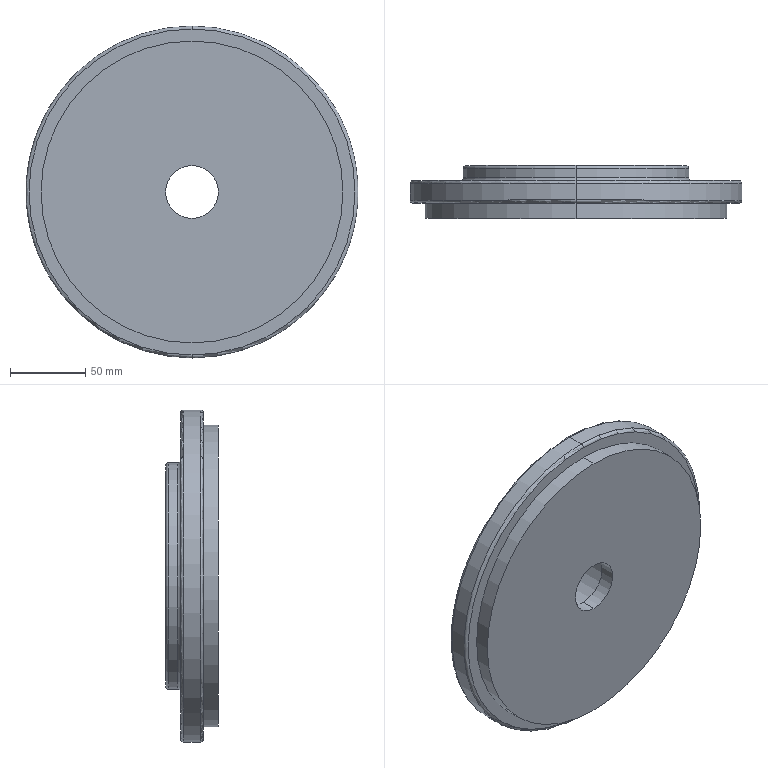Part | SolidWorks | features ICE 4, Fillet 2, CirPattern 1, Extrusion 1, HoleWzd 1 | 1 solid | 39 faces | box 220 x 35 x 220 mm | volume 996825 mm3 | cylinder 18 | torus 8 | cone 8 | plane 5 | commonest cylinder face diameters 3.3 x8 35 x2 52 x2 150 x2 200 x2 220 x2
STEP:
#1=CARTESIAN_POINT('',(0.,23.,-110.));
#2=VERTEX_POINT('',#1);
#3=CARTESIAN_POINT('',(0.,23.,110.));
#4=VERTEX_POINT('',#3);
#5=CARTESIAN_POINT('',(0.,23.,0.));
#6=DIRECTION('',(0.,-1.,0.));
#7=DIRECTION('',(0.,0.,1.));
#8=AXIS2_PLACEMENT_3D('',#5,#6,#7);
#9=CIRCLE('',#8,110.);
#10=EDGE_CURVE('',#2,#4,#9,.T.);
#11=ORIENTED_EDGE('',*,*,#10,.F.);
#12=CARTESIAN_POINT('',(0.,25.,-108.));
#13=VERTEX_POINT('',#12);
#14=CARTESIAN_POINT('',(0.,23.,-108.));
#15=DIRECTION('',(1.,0.,0.));
#16=DIRECTION('',(0.,0.,-1.));
#17=AXIS2_PLACEMENT_3D('',#14,#15,#16);
#18=CIRCLE('',#17,2.);
#19=EDGE_CURVE('',#2,#13,#18,.T.);
#20=ORIENTED_EDGE('',*,*,#19,.T.);
#21=CARTESIAN_POINT('',(0.,25.,108.));
#22=VERTEX_POINT('',#21);
#23=CARTESIAN_POINT('',(0.,25.,0.));
#24=DIRECTION('',(0.,1.,0.));
#25=DIRECTION('',(0.,0.,1.));
#26=AXIS2_PLACEMENT_3D('',#23,#24,#25);
#27=CIRCLE('',#26,108.);
#28=EDGE_CURVE('',#22,#13,#27,.T.);
#29=ORIENTED_EDGE('',*,*,#28,.F.);
#30=CARTESIAN_POINT('',(0.,23.,108.));
#31=DIRECTION('',(-1.,0.,0.));
#32=DIRECTION('',(0.,0.,1.));
#33=AXIS2_PLACEMENT_3D('',#30,#31,#32);
#34=CIRCLE('',#33,2.);
#35=EDGE_CURVE('',#4,#22,#34,.T.);
#36=ORIENTED_EDGE('',*,*,#35,.F.);
#37=EDGE_LOOP('',(#11,#20,#29,#36));
#38=FACE_OUTER_BOUND('',#37,.T.);
#39=CARTESIAN_POINT('',(0.,23.,0.));
#40=DIRECTION('',(0.,1.,0.));
#41=DIRECTION('',(0.,0.,1.));
#42=AXIS2_PLACEMENT_3D('',#39,#40,#41);
#43=TOROIDAL_SURFACE('',#42,108.,2.);
#44=ADVANCED_FACE('',(#38),#43,.T.);
#45=CARTESIAN_POINT('',(0.,10.,-108.));
#46=VERTEX_POINT('',#45);
#47=CARTESIAN_POINT('',(0.,10.,108.));
#48=VERTEX_POINT('',#47);
#49=CARTESIAN_POINT('',(0.,10.,0.));
#50=DIRECTION('',(0.,-1.,0.));
#51=DIRECTION('',(0.,0.,1.));
#52=AXIS2_PLACEMENT_3D('',#49,#50,#51);
#53=CIRCLE('',#52,108.);
#54=EDGE_CURVE('',#46,#48,#53,.T.);
#55=ORIENTED_EDGE('',*,*,#54,.F.);
#56=CARTESIAN_POINT('',(0.,12.,-110.));
#57=VERTEX_POINT('',#56);
#58=CARTESIAN_POINT('',(0.,12.,-108.));
#59=DIRECTION('',(1.,0.,0.));
#60=DIRECTION('',(0.,0.,-1.));
#61=AXIS2_PLACEMENT_3D('',#58,#59,#60);
#62=CIRCLE('',#61,2.);
#63=EDGE_CURVE('',#46,#57,#62,.T.);
#64=ORIENTED_EDGE('',*,*,#63,.T.);
#65=CARTESIAN_POINT('',(0.,12.,110.));
#66=VERTEX_POINT('',#65);
#67=CARTESIAN_POINT('',(0.,12.,0.));
#68=DIRECTION('',(0.,1.,0.));
#69=DIRECTION('',(0.,0.,1.));
#70=AXIS2_PLACEMENT_3D('',#67,#68,#69);
#71=CIRCLE('',#70,110.);
#72=EDGE_CURVE('',#66,#57,#71,.T.);
#73=ORIENTED_EDGE('',*,*,#72,.F.);
#74=CARTESIAN_POINT('',(0.,12.,108.));
#75=DIRECTION('',(-1.,0.,0.));
#76=DIRECTION('',(0.,0.,1.));
#77=AXIS2_PLACEMENT_3D('',#74,#75,#76);
#78=CIRCLE('',#77,2.);
#79=EDGE_CURVE('',#48,#66,#78,.T.);
#80=ORIENTED_EDGE('',*,*,#79,.F.);
#81=EDGE_LOOP('',(#55,#64,#73,#80));
#82=FACE_OUTER_BOUND('',#81,.T.);
#83=CARTESIAN_POINT('',(0.,12.,0.));
#84=DIRECTION('',(0.,1.,0.));
#85=DIRECTION('',(0.,0.,1.));
#86=AXIS2_PLACEMENT_3D('',#83,#84,#85);
#87=TOROIDAL_SURFACE('',#86,108.,2.);
#88=ADVANCED_FACE('',(#82),#87,.T.);
#89=CARTESIAN_POINT('',(30.,24.9,-1.65));
#90=VERTEX_POINT('',#89);
#91=CARTESIAN_POINT('',(30.,24.9,1.65));
#92=VERTEX_POINT('',#91);
#93=CARTESIAN_POINT('',(30.,24.9,0.));
#94=DIRECTION('',(0.,1.,0.));
#95=DIRECTION('',(0.,0.,1.));
#96=AXIS2_PLACEMENT_3D('',#93,#94,#95);
#97=CIRCLE('',#96,1.65);
#98=EDGE_CURVE('',#90,#92,#97,.T.);
#99=ORIENTED_EDGE('',*,*,#98,.F.);
#100=CARTESIAN_POINT('',(30.,35.,-1.65));
#101=VERTEX_POINT('',#100);
#102=CARTESIAN_POINT('',(30.,35.,-1.65));
#103=DIRECTION('',(0.,1.,0.));
#104=VECTOR('',#103,1000.);
#105=LINE('',#102,#104);
#106=EDGE_CURVE('',#90,#101,#105,.T.);
#107=ORIENTED_EDGE('',*,*,#106,.T.);
#108=CARTESIAN_POINT('',(30.,35.,1.65));
#109=VERTEX_POINT('',#108);
#110=CARTESIAN_POINT('',(30.,35.,0.));
#111=DIRECTION('',(0.,1.,0.));
#112=DIRECTION('',(0.,0.,1.));
#113=AXIS2_PLACEMENT_3D('',#110,#111,#112);
#114=CIRCLE('',#113,1.65);
#115=EDGE_CURVE('',#101,#109,#114,.T.);
#116=ORIENTED_EDGE('',*,*,#115,.T.);
#117=CARTESIAN_POINT('',(30.,35.,1.65));
#118=DIRECTION('',(0.,1.,0.));
#119=VECTOR('',#118,1000.);
#120=LINE('',#117,#119);
#121=EDGE_CURVE('',#92,#109,#120,.T.);
#122=ORIENTED_EDGE('',*,*,#121,.F.);
#123=EDGE_LOOP('',(#99,#107,#116,#122));
#124=FACE_OUTER_BOUND('',#123,.T.);
#125=CARTESIAN_POINT('',(30.,35.,0.));
#126=DIRECTION('',(0.,1.,0.));
#127=DIRECTION('',(0.,0.,1.));
#128=AXIS2_PLACEMENT_3D('',#125,#126,#127);
#129=CYLINDRICAL_SURFACE('',#128,1.65);
#130=ADVANCED_FACE('',(#124),#129,.F.);
#131=CARTESIAN_POINT('',(30.,23.909,0.));
#132=VERTEX_POINT('',#131);
#133=CARTESIAN_POINT('',(30.,24.9,1.65));
#134=DIRECTION('',(0.,0.515,0.8572));
#135=VECTOR('',#134,1000.);
#136=LINE('',#133,#135);
#137=EDGE_CURVE('',#132,#92,#136,.T.);
#138=ORIENTED_EDGE('',*,*,#137,.F.);
#139=CARTESIAN_POINT('',(30.,24.9,-1.65));
#140=DIRECTION('',(0.,0.515,-0.8572));
#141=VECTOR('',#140,1000.);
#142=LINE('',#139,#141);
#143=EDGE_CURVE('',#132,#90,#142,.T.);
#144=ORIENTED_EDGE('',*,*,#143,.T.);
#145=ORIENTED_EDGE('',*,*,#98,.T.);
#146=EDGE_LOOP('',(#138,#144,#145));
#147=FACE_OUTER_BOUND('',#146,.T.);
#148=CARTESIAN_POINT('',(30.,24.9,0.));
#149=DIRECTION('',(0.,1.,0.));
#150=DIRECTION('',(0.,0.,1.));
#151=AXIS2_PLACEMENT_3D('',#148,#149,#150);
#152=CONICAL_SURFACE('',#151,1.65,1.03);
#153=ADVANCED_FACE('',(#147),#152,.F.);
#154=CARTESIAN_POINT('',(0.,24.9,28.35));
#155=VERTEX_POINT('',#154);
#156=CARTESIAN_POINT('',(0.,24.9,31.65));
#157=VERTEX_POINT('',#156);
#158=CARTESIAN_POINT('',(0.,24.9,30.));
#159=DIRECTION('',(0.,1.,0.));
#160=DIRECTION('',(0.,0.,1.));
#161=AXIS2_PLACEMENT_3D('',#158,#159,#160);
#162=CIRCLE('',#161,1.65);
#163=EDGE_CURVE('',#155,#157,#162,.T.);
#164=ORIENTED_EDGE('',*,*,#163,.F.);
#165=CARTESIAN_POINT('',(0.,35.,28.35));
#166=VERTEX_POINT('',#165);
#167=CARTESIAN_POINT('',(0.,35.,28.35));
#168=DIRECTION('',(0.,1.,0.));
#169=VECTOR('',#168,1000.);
#170=LINE('',#167,#169);
#171=EDGE_CURVE('',#155,#166,#170,.T.);
#172=ORIENTED_EDGE('',*,*,#171,.T.);
#173=CARTESIAN_POINT('',(0.,35.,31.65));
#174=VERTEX_POINT('',#173);
#175=CARTESIAN_POINT('',(0.,35.,30.));
#176=DIRECTION('',(0.,1.,0.));
#177=DIRECTION('',(0.,0.,1.));
#178=AXIS2_PLACEMENT_3D('',#175,#176,#177);
#179=CIRCLE('',#178,1.65);
#180=EDGE_CURVE('',#166,#174,#179,.T.);
#181=ORIENTED_EDGE('',*,*,#180,.T.);
#182=CARTESIAN_POINT('',(0.,35.,31.65));
#183=DIRECTION('',(0.,1.,0.));
#184=VECTOR('',#183,1000.);
#185=LINE('',#182,#184);
#186=EDGE_CURVE('',#157,#174,#185,.T.);
#187=ORIENTED_EDGE('',*,*,#186,.F.);
#188=EDGE_LOOP('',(#164,#172,#181,#187));
#189=FACE_OUTER_BOUND('',#188,.T.);
#190=CARTESIAN_POINT('',(0.,35.,30.));
#191=DIRECTION('',(0.,1.,0.));
#192=DIRECTION('',(0.,0.,1.));
#193=AXIS2_PLACEMENT_3D('',#190,#191,#192);
#194=CYLINDRICAL_SURFACE('',#193,1.65);
#195=ADVANCED_FACE('',(#189),#194,.F.);
#196=CARTESIAN_POINT('',(0.,23.909,30.));
#197=VERTEX_POINT('',#196);
#198=CARTESIAN_POINT('',(0.,24.9,31.65));
#199=DIRECTION('',(0.,0.515,0.8572));
#200=VECTOR('',#199,1000.);
#201=LINE('',#198,#200);
#202=EDGE_CURVE('',#197,#157,#201,.T.);
#203=ORIENTED_EDGE('',*,*,#202,.F.);
#204=CARTESIAN_POINT('',(0.,24.9,28.35));
#205=DIRECTION('',(0.,0.515,-0.8572));
#206=VECTOR('',#205,1000.);
#207=LINE('',#204,#206);
#208=EDGE_CURVE('',#197,#155,#207,.T.);
#209=ORIENTED_EDGE('',*,*,#208,.T.);
#210=ORIENTED_EDGE('',*,*,#163,.T.);
#211=EDGE_LOOP('',(#203,#209,#210));
#212=FACE_OUTER_BOUND('',#211,.T.);
#213=CARTESIAN_POINT('',(0.,24.9,30.));
#214=DIRECTION('',(0.,1.,0.));
#215=DIRECTION('',(0.,0.,1.));
#216=AXIS2_PLACEMENT_3D('',#213,#214,#215);
#217=CONICAL_SURFACE('',#216,1.65,1.03);
#218=ADVANCED_FACE('',(#212),#217,.F.);
#219=CARTESIAN_POINT('',(-30.,24.9,-1.65));
#220=VERTEX_POINT('',#219);
#221=CARTESIAN_POINT('',(-30.,24.9,1.65));
#222=VERTEX_POINT('',#221);
#223=CARTESIAN_POINT('',(-30.,24.9,0.));
#224=DIRECTION('',(0.,1.,0.));
#225=DIRECTION('',(0.,0.,1.));
#226=AXIS2_PLACEMENT_3D('',#223,#224,#225);
#227=CIRCLE('',#226,1.65);
#228=EDGE_CURVE('',#220,#222,#227,.T.);
#229=ORIENTED_EDGE('',*,*,#228,.F.);
#230=CARTESIAN_POINT('',(-30.,35.,-1.65));
#231=VERTEX_POINT('',#230);
#232=CARTESIAN_POINT('',(-30.,35.,-1.65));
#233=DIRECTION('',(0.,1.,0.));
#234=VECTOR('',#233,1000.);
#235=LINE('',#232,#234);
#236=EDGE_CURVE('',#220,#231,#235,.T.);
#237=ORIENTED_EDGE('',*,*,#236,.T.);
#238=CARTESIAN_POINT('',(-30.,35.,1.65));
#239=VERTEX_POINT('',#238);
#240=CARTESIAN_POINT('',(-30.,35.,0.));
#241=DIRECTION('',(0.,1.,0.));
#242=DIRECTION('',(0.,0.,1.));
#243=AXIS2_PLACEMENT_3D('',#240,#241,#242);
#244=CIRCLE('',#243,1.65);
#245=EDGE_CURVE('',#231,#239,#244,.T.);
#246=ORIENTED_EDGE('',*,*,#245,.T.);
#247=CARTESIAN_POINT('',(-30.,35.,1.65));
#248=DIRECTION('',(0.,1.,0.));
#249=VECTOR('',#248,1000.);
#250=LINE('',#247,#249);
#251=EDGE_CURVE('',#222,#239,#250,.T.);
#252=ORIENTED_EDGE('',*,*,#251,.F.);
#253=EDGE_LOOP('',(#229,#237,#246,#252));
#254=FACE_OUTER_BOUND('',#253,.T.);
#255=CARTESIAN_POINT('',(-30.,35.,0.));
#256=DIRECTION('',(0.,1.,0.));
#257=DIRECTION('',(0.,0.,1.));
#258=AXIS2_PLACEMENT_3D('',#255,#256,#257);
#259=CYLINDRICAL_SURFACE('',#258,1.65);
#260=ADVANCED_FACE('',(#254),#259,.F.);
#261=CARTESIAN_POINT('',(-30.,23.909,0.));
#262=VERTEX_POINT('',#261);
#263=CARTESIAN_POINT('',(-30.,24.9,1.65));
#264=DIRECTION('',(0.,0.515,0.8572));
#265=VECTOR('',#264,1000.);
#266=LINE('',#263,#265);
#267=EDGE_CURVE('',#262,#222,#266,.T.);
#268=ORIENTED_EDGE('',*,*,#267,.F.);
#269=CARTESIAN_POINT('',(-30.,24.9,-1.65));
#270=DIRECTION('',(0.,0.515,-0.8572));
#271=VECTOR('',#270,1000.);
#272=LINE('',#269,#271);
#273=EDGE_CURVE('',#262,#220,#272,.T.);
#274=ORIENTED_EDGE('',*,*,#273,.T.);
#275=ORIENTED_EDGE('',*,*,#228,.T.);
#276=EDGE_LOOP('',(#268,#274,#275));
#277=FACE_OUTER_BOUND('',#276,.T.);
#278=CARTESIAN_POINT('',(-30.,24.9,0.));
#279=DIRECTION('',(0.,1.,0.));
#280=DIRECTION('',(0.,0.,1.));
#281=AXIS2_PLACEMENT_3D('',#278,#279,#280);
#282=CONICAL_SURFACE('',#281,1.65,1.03);
#283=ADVANCED_FACE('',(#277),#282,.F.);
#284=CARTESIAN_POINT('',(0.,24.9,-31.65));
#285=VERTEX_POINT('',#284);
#286=CARTESIAN_POINT('',(0.,24.9,-28.35));
#287=VERTEX_POINT('',#286);
#288=CARTESIAN_POINT('',(0.,24.9,-30.));
#289=DIRECTION('',(0.,1.,0.));
#290=DIRECTION('',(0.,0.,1.));
#291=AXIS2_PLACEMENT_3D('',#288,#289,#290);
#292=CIRCLE('',#291,1.65);
#293=EDGE_CURVE('',#285,#287,#292,.T.);
#294=ORIENTED_EDGE('',*,*,#293,.F.);
#295=CARTESIAN_POINT('',(0.,35.,-31.65));
#296=VERTEX_POINT('',#295);
#297=CARTESIAN_POINT('',(0.,35.,-31.65));
#298=DIRECTION('',(0.,1.,0.));
#299=VECTOR('',#298,1000.);
#300=LINE('',#297,#299);
#301=EDGE_CURVE('',#285,#296,#300,.T.);
#302=ORIENTED_EDGE('',*,*,#301,.T.);
#303=CARTESIAN_POINT('',(0.,35.,-28.35));
#304=VERTEX_POINT('',#303);
#305=CARTESIAN_POINT('',(0.,35.,-30.));
#306=DIRECTION('',(0.,1.,0.));
#307=DIRECTION('',(0.,0.,1.));
#308=AXIS2_PLACEMENT_3D('',#305,#306,#307);
#309=CIRCLE('',#308,1.65);
#310=EDGE_CURVE('',#296,#304,#309,.T.);
#311=ORIENTED_EDGE('',*,*,#310,.T.);
#312=CARTESIAN_POINT('',(0.,35.,-28.35));
#313=DIRECTION('',(0.,1.,0.));
#314=VECTOR('',#313,1000.);
#315=LINE('',#312,#314);
#316=EDGE_CURVE('',#287,#304,#315,.T.);
#317=ORIENTED_EDGE('',*,*,#316,.F.);
#318=EDGE_LOOP('',(#294,#302,#311,#317));
#319=FACE_OUTER_BOUND('',#318,.T.);
#320=CARTESIAN_POINT('',(0.,35.,-30.));
#321=DIRECTION('',(0.,1.,0.));
#322=DIRECTION('',(0.,0.,1.));
#323=AXIS2_PLACEMENT_3D('',#320,#321,#322);
#324=CYLINDRICAL_SURFACE('',#323,1.65);
#325=ADVANCED_FACE('',(#319),#324,.F.);
#326=CARTESIAN_POINT('',(0.,23.909,-30.));
#327=VERTEX_POINT('',#326);
#328=CARTESIAN_POINT('',(0.,24.9,-28.35));
#329=DIRECTION('',(0.,0.515,0.8572));
#330=VECTOR('',#329,1000.);
#331=LINE('',#328,#330);
#332=EDGE_CURVE('',#327,#287,#331,.T.);
#333=ORIENTED_EDGE('',*,*,#332,.F.);
#334=CARTESIAN_POINT('',(0.,24.9,-31.65));
#335=DIRECTION('',(0.,0.515,-0.8572));
#336=VECTOR('',#335,1000.);
#337=LINE('',#334,#336);
#338=EDGE_CURVE('',#327,#285,#337,.T.);
#339=ORIENTED_EDGE('',*,*,#338,.T.);
#340=ORIENTED_EDGE('',*,*,#293,.T.);
#341=EDGE_LOOP('',(#333,#339,#340));
#342=FACE_OUTER_BOUND('',#341,.T.);
#343=CARTESIAN_POINT('',(0.,24.9,-30.));
#344=DIRECTION('',(0.,1.,0.));
#345=DIRECTION('',(0.,0.,1.));
#346=AXIS2_PLACEMENT_3D('',#343,#344,#345);
#347=CONICAL_SURFACE('',#346,1.65,1.03);
#348=ADVANCED_FACE('',(#342),#347,.F.);
#349=CARTESIAN_POINT('',(0.,0.,-17.5));
#350=VERTEX_POINT('',#349);
#351=CARTESIAN_POINT('',(0.,0.,17.5));
#352=VERTEX_POINT('',#351);
#353=CARTESIAN_POINT('',(0.,0.,0.));
#354=DIRECTION('',(0.,1.,0.));
#355=DIRECTION('',(0.,0.,1.));
#356=AXIS2_PLACEMENT_3D('',#353,#354,#355);
#357=CIRCLE('',#356,17.5);
#358=EDGE_CURVE('',#350,#352,#357,.T.);
#359=ORIENTED_EDGE('',*,*,#358,.F.);
#360=CARTESIAN_POINT('',(0.,10.,-17.5));
#361=VERTEX_POINT('',#360);
#362=CARTESIAN_POINT('',(0.,0.,-17.5));
#363=DIRECTION('',(0.,1.,0.));
#364=VECTOR('',#363,1000.);
#365=LINE('',#362,#364);
#366=EDGE_CURVE('',#350,#361,#365,.T.);
#367=ORIENTED_EDGE('',*,*,#366,.T.);
#368=CARTESIAN_POINT('',(0.,10.,17.5));
#369=VERTEX_POINT('',#368);
#370=CARTESIAN_POINT('',(0.,10.,0.));
#371=DIRECTION('',(0.,1.,0.));
#372=DIRECTION('',(0.,0.,1.));
#373=AXIS2_PLACEMENT_3D('',#370,#371,#372);
#374=CIRCLE('',#373,17.5);
#375=EDGE_CURVE('',#361,#369,#374,.T.);
#376=ORIENTED_EDGE('',*,*,#375,.T.);
#377=CARTESIAN_POINT('',(0.,0.,17.5));
#378=DIRECTION('',(0.,1.,0.));
#379=VECTOR('',#378,1000.);
#380=LINE('',#377,#379);
#381=EDGE_CURVE('',#352,#369,#380,.T.);
#382=ORIENTED_EDGE('',*,*,#381,.F.);
#383=EDGE_LOOP('',(#359,#367,#376,#382));
#384=FACE_OUTER_BOUND('',#383,.T.);
#385=CARTESIAN_POINT('',(0.,0.,0.));
#386=DIRECTION('',(0.,1.,0.));
#387=DIRECTION('',(0.,0.,1.));
#388=AXIS2_PLACEMENT_3D('',#385,#386,#387);
#389=CYLINDRICAL_SURFACE('',#388,17.5);
#390=ADVANCED_FACE('',(#384),#389,.F.);
#391=CARTESIAN_POINT('',(0.,10.,-26.));
#392=VERTEX_POINT('',#391);
#393=CARTESIAN_POINT('',(0.,10.,26.));
#394=VERTEX_POINT('',#393);
#395=CARTESIAN_POINT('',(0.,10.,0.));
#396=DIRECTION('',(0.,1.,0.));
#397=DIRECTION('',(0.,0.,1.));
#398=AXIS2_PLACEMENT_3D('',#395,#396,#397);
#399=CIRCLE('',#398,26.);
#400=EDGE_CURVE('',#392,#394,#399,.T.);
#401=ORIENTED_EDGE('',*,*,#400,.F.);
#402=CARTESIAN_POINT('',(0.,35.,-26.));
#403=VERTEX_POINT('',#402);
#404=CARTESIAN_POINT('',(0.,10.,-26.));
#405=DIRECTION('',(0.,1.,0.));
#406=VECTOR('',#405,1000.);
#407=LINE('',#404,#406);
#408=EDGE_CURVE('',#392,#403,#407,.T.);
#409=ORIENTED_EDGE('',*,*,#408,.T.);
#410=CARTESIAN_POINT('',(0.,35.,26.));
#411=VERTEX_POINT('',#410);
#412=CARTESIAN_POINT('',(0.,35.,0.));
#413=DIRECTION('',(0.,1.,0.));
#414=DIRECTION('',(0.,0.,1.));
#415=AXIS2_PLACEMENT_3D('',#412,#413,#414);
#416=CIRCLE('',#415,26.);
#417=EDGE_CURVE('',#403,#411,#416,.T.);
#418=ORIENTED_EDGE('',*,*,#417,.T.);
#419=CARTESIAN_POINT('',(0.,10.,26.));
#420=DIRECTION('',(0.,1.,0.));
#421=VECTOR('',#420,1000.);
#422=LINE('',#419,#421);
#423=EDGE_CURVE('',#394,#411,#422,.T.);
#424=ORIENTED_EDGE('',*,*,#423,.F.);
#425=EDGE_LOOP('',(#401,#409,#418,#424));
#426=FACE_OUTER_BOUND('',#425,.T.);
#427=CARTESIAN_POINT('',(0.,10.,0.));
#428=DIRECTION('',(0.,1.,0.));
#429=DIRECTION('',(0.,0.,1.));
#430=AXIS2_PLACEMENT_3D('',#427,#428,#429);
#431=CYLINDRICAL_SURFACE('',#430,26.);
#432=ADVANCED_FACE('',(#426),#431,.F.);
#433=CARTESIAN_POINT('',(0.,27.,-75.));
#434=VERTEX_POINT('',#433);
#435=CARTESIAN_POINT('',(0.,27.,75.));
#436=VERTEX_POINT('',#435);
#437=CARTESIAN_POINT('',(0.,27.,0.));
#438=DIRECTION('',(0.,1.,0.));
#439=DIRECTION('',(0.,0.,1.));
#440=AXIS2_PLACEMENT_3D('',#437,#438,#439);
#441=CIRCLE('',#440,75.);
#442=EDGE_CURVE('',#434,#436,#441,.T.);
#443=ORIENTED_EDGE('',*,*,#442,.F.);
#444=CARTESIAN_POINT('',(0.,25.,-77.));
#445=VERTEX_POINT('',#444);
#446=CARTESIAN_POINT('',(0.,27.,-77.));
#447=DIRECTION('',(1.,0.,0.));
#448=DIRECTION('',(0.,0.,-1.));
#449=AXIS2_PLACEMENT_3D('',#446,#447,#448);
#450=CIRCLE('',#449,2.);
#451=EDGE_CURVE('',#434,#445,#450,.T.);
#452=ORIENTED_EDGE('',*,*,#451,.T.);
#453=CARTESIAN_POINT('',(0.,25.,77.));
#454=VERTEX_POINT('',#453);
#455=CARTESIAN_POINT('',(0.,25.,0.));
#456=DIRECTION('',(0.,-1.,0.));
#457=DIRECTION('',(0.,0.,1.));
#458=AXIS2_PLACEMENT_3D('',#455,#456,#457);
#459=CIRCLE('',#458,77.);
#460=EDGE_CURVE('',#454,#445,#459,.T.);
#461=ORIENTED_EDGE('',*,*,#460,.F.);
#462=CARTESIAN_POINT('',(0.,27.,77.));
#463=DIRECTION('',(-1.,0.,0.));
#464=DIRECTION('',(0.,0.,1.));
#465=AXIS2_PLACEMENT_3D('',#462,#463,#464);
#466=CIRCLE('',#465,2.);
#467=EDGE_CURVE('',#436,#454,#466,.T.);
#468=ORIENTED_EDGE('',*,*,#467,.F.);
#469=EDGE_LOOP('',(#443,#452,#461,#468));
#470=FACE_OUTER_BOUND('',#469,.T.);
#471=CARTESIAN_POINT('',(0.,27.,0.));
#472=DIRECTION('',(0.,1.,0.));
#473=DIRECTION('',(0.,0.,1.));
#474=AXIS2_PLACEMENT_3D('',#471,#472,#473);
#475=TOROIDAL_SURFACE('',#474,77.,2.);
#476=ADVANCED_FACE('',(#470),#475,.F.);
#477=CARTESIAN_POINT('',(0.,33.,-75.));
#478=VERTEX_POINT('',#477);
#479=CARTESIAN_POINT('',(0.,33.,75.));
#480=VERTEX_POINT('',#479);
#481=CARTESIAN_POINT('',(0.,33.,0.));
#482=DIRECTION('',(0.,-1.,0.));
#483=DIRECTION('',(0.,0.,1.));
#484=AXIS2_PLACEMENT_3D('',#481,#482,#483);
#485=CIRCLE('',#484,75.);
#486=EDGE_CURVE('',#478,#480,#485,.T.);
#487=ORIENTED_EDGE('',*,*,#486,.F.);
#488=CARTESIAN_POINT('',(0.,35.,-73.));
#489=VERTEX_POINT('',#488);
#490=CARTESIAN_POINT('',(0.,33.,-73.));
#491=DIRECTION('',(1.,0.,0.));
#492=DIRECTION('',(0.,0.,-1.));
#493=AXIS2_PLACEMENT_3D('',#490,#491,#492);
#494=CIRCLE('',#493,2.);
#495=EDGE_CURVE('',#478,#489,#494,.T.);
#496=ORIENTED_EDGE('',*,*,#495,.T.);
#497=CARTESIAN_POINT('',(0.,35.,73.));
#498=VERTEX_POINT('',#497);
#499=CARTESIAN_POINT('',(0.,35.,0.));
#500=DIRECTION('',(0.,1.,0.));
#501=DIRECTION('',(0.,0.,1.));
#502=AXIS2_PLACEMENT_3D('',#499,#500,#501);
#503=CIRCLE('',#502,73.);
#504=EDGE_CURVE('',#498,#489,#503,.T.);
#505=ORIENTED_EDGE('',*,*,#504,.F.);
#506=CARTESIAN_POINT('',(0.,33.,73.));
#507=DIRECTION('',(-1.,0.,0.));
#508=DIRECTION('',(0.,0.,1.));
#509=AXIS2_PLACEMENT_3D('',#506,#507,#508);
#510=CIRCLE('',#509,2.);
#511=EDGE_CURVE('',#480,#498,#510,.T.);
#512=ORIENTED_EDGE('',*,*,#511,.F.);
#513=EDGE_LOOP('',(#487,#496,#505,#512));
#514=FACE_OUTER_BOUND('',#513,.T.);
#515=CARTESIAN_POINT('',(0.,33.,0.));
#516=DIRECTION('',(0.,1.,0.));
#517=DIRECTION('',(0.,0.,1.));
#518=AXIS2_PLACEMENT_3D('',#515,#516,#517);
#519=TOROIDAL_SURFACE('',#518,73.,2.);
#520=ADVANCED_FACE('',(#514),#519,.T.);
#521=ORIENTED_EDGE('',*,*,#486,.T.);
#522=CARTESIAN_POINT('',(0.,35.,75.));
#523=DIRECTION('',(0.,-1.,0.));
#524=VECTOR('',#523,1000.);
#525=LINE('',#522,#524);
#526=EDGE_CURVE('',#480,#436,#525,.T.);
#527=ORIENTED_EDGE('',*,*,#526,.T.);
#528=CARTESIAN_POINT('',(0.,27.,0.));
#529=DIRECTION('',(0.,1.,0.));
#530=DIRECTION('',(0.,0.,1.));
#531=AXIS2_PLACEMENT_3D('',#528,#529,#530);
#532=CIRCLE('',#531,75.);
#533=EDGE_CURVE('',#436,#434,#532,.T.);
#534=ORIENTED_EDGE('',*,*,#533,.T.);
#535=CARTESIAN_POINT('',(0.,35.,-75.));
#536=DIRECTION('',(0.,-1.,0.));
#537=VECTOR('',#536,1000.);
#538=LINE('',#535,#537);
#539=EDGE_CURVE('',#478,#434,#538,.T.);
#540=ORIENTED_EDGE('',*,*,#539,.F.);
#541=EDGE_LOOP('',(#521,#527,#534,#540));
#542=FACE_OUTER_BOUND('',#541,.T.);
#543=CARTESIAN_POINT('',(0.,35.,0.));
#544=DIRECTION('',(0.,-1.,0.));
#545=DIRECTION('',(0.,0.,-1.));
#546=AXIS2_PLACEMENT_3D('',#543,#544,#545);
#547=CYLINDRICAL_SURFACE('',#546,75.);
#548=ADVANCED_FACE('',(#542),#547,.T.);
#549=ORIENTED_EDGE('',*,*,#10,.T.);
#550=CARTESIAN_POINT('',(0.,25.,110.));
#551=DIRECTION('',(0.,-1.,0.));
#552=VECTOR('',#551,1000.);
#553=LINE('',#550,#552);
#554=EDGE_CURVE('',#4,#66,#553,.T.);
#555=ORIENTED_EDGE('',*,*,#554,.T.);
#556=ORIENTED_EDGE('',*,*,#72,.T.);
#557=CARTESIAN_POINT('',(0.,25.,-110.));
#558=DIRECTION('',(0.,-1.,0.));
#559=VECTOR('',#558,1000.);
#560=LINE('',#557,#559);
#561=EDGE_CURVE('',#2,#57,#560,.T.);
#562=ORIENTED_EDGE('',*,*,#561,.F.);
#563=EDGE_LOOP('',(#549,#555,#556,#562));
#564=FACE_OUTER_BOUND('',#563,.T.);
#565=CARTESIAN_POINT('',(0.,25.,0.));
#566=DIRECTION('',(0.,-1.,0.));
#567=DIRECTION('',(0.,0.,-1.));
#568=AXIS2_PLACEMENT_3D('',#565,#566,#567);
#569=CYLINDRICAL_SURFACE('',#568,110.);
#570=ADVANCED_FACE('',(#564),#569,.T.);
#571=CARTESIAN_POINT('',(0.,10.,100.));
#572=VERTEX_POINT('',#571);
#573=CARTESIAN_POINT('',(0.,10.,-100.));
#574=VERTEX_POINT('',#573);
#575=CARTESIAN_POINT('',(0.,10.,0.));
#576=DIRECTION('',(0.,1.,0.));
#577=DIRECTION('',(0.,0.,1.));
#578=AXIS2_PLACEMENT_3D('',#575,#576,#577);
#579=CIRCLE('',#578,100.);
#580=EDGE_CURVE('',#572,#574,#579,.T.);
#581=ORIENTED_EDGE('',*,*,#580,.F.);
#582=CARTESIAN_POINT('',(0.,0.,100.));
#583=VERTEX_POINT('',#582);
#584=CARTESIAN_POINT('',(0.,10.,100.));
#585=DIRECTION('',(0.,-1.,0.));
#586=VECTOR('',#585,1000.);
#587=LINE('',#584,#586);
#588=EDGE_CURVE('',#572,#583,#587,.T.);
#589=ORIENTED_EDGE('',*,*,#588,.T.);
#590=CARTESIAN_POINT('',(0.,0.,-100.));
#591=VERTEX_POINT('',#590);
#592=CARTESIAN_POINT('',(0.,0.,0.));
#593=DIRECTION('',(0.,1.,0.));
#594=DIRECTION('',(0.,0.,1.));
#595=AXIS2_PLACEMENT_3D('',#592,#593,#594);
#596=CIRCLE('',#595,100.);
#597=EDGE_CURVE('',#583,#591,#596,.T.);
#598=ORIENTED_EDGE('',*,*,#597,.T.);
#599=CARTESIAN_POINT('',(0.,10.,-100.));
#600=DIRECTION('',(0.,-1.,0.));
#601=VECTOR('',#600,1000.);
#602=LINE('',#599,#601);
#603=EDGE_CURVE('',#574,#591,#602,.T.);
#604=ORIENTED_EDGE('',*,*,#603,.F.);
#605=EDGE_LOOP('',(#581,#589,#598,#604));
#606=FACE_OUTER_BOUND('',#605,.T.);
#607=CARTESIAN_POINT('',(0.,10.,0.));
#608=DIRECTION('',(0.,-1.,0.));
#609=DIRECTION('',(0.,0.,-1.));
#610=AXIS2_PLACEMENT_3D('',#607,#608,#609);
#611=CYLINDRICAL_SURFACE('',#610,100.);
#612=ADVANCED_FACE('',(#606),#611,.T.);
#613=ORIENTED_EDGE('',*,*,#588,.F.);
#614=CARTESIAN_POINT('',(0.,10.,0.));
#615=DIRECTION('',(0.,1.,0.));
#616=DIRECTION('',(0.,0.,1.));
#617=AXIS2_PLACEMENT_3D('',#614,#615,#616);
#618=CIRCLE('',#617,100.);
#619=EDGE_CURVE('',#574,#572,#618,.T.);
#620=ORIENTED_EDGE('',*,*,#619,.F.);
#621=ORIENTED_EDGE('',*,*,#603,.T.);
#622=CARTESIAN_POINT('',(0.,0.,0.));
#623=DIRECTION('',(0.,1.,0.));
#624=DIRECTION('',(0.,0.,1.));
#625=AXIS2_PLACEMENT_3D('',#622,#623,#624);
#626=CIRCLE('',#625,100.);
#627=EDGE_CURVE('',#591,#583,#626,.T.);
#628=ORIENTED_EDGE('',*,*,#627,.T.);
#629=EDGE_LOOP('',(#613,#620,#621,#628));
#630=FACE_OUTER_BOUND('',#629,.T.);
#631=CARTESIAN_POINT('',(0.,10.,0.));
#632=DIRECTION('',(0.,-1.,0.));
#633=DIRECTION('',(0.,0.,-1.));
#634=AXIS2_PLACEMENT_3D('',#631,#632,#633);
#635=CYLINDRICAL_SURFACE('',#634,100.);
#636=ADVANCED_FACE('',(#630),#635,.T.);
#637=CARTESIAN_POINT('',(0.,0.,0.));
#638=DIRECTION('',(0.,1.,0.));
#639=DIRECTION('',(0.,0.,1.));
#640=AXIS2_PLACEMENT_3D('',#637,#638,#639);
#641=CIRCLE('',#640,17.5);
#642=EDGE_CURVE('',#352,#350,#641,.T.);
#643=ORIENTED_EDGE('',*,*,#642,.T.);
#644=ORIENTED_EDGE('',*,*,#358,.T.);
#645=EDGE_LOOP('',(#643,#644));
#646=FACE_BOUND('',#645,.T.);
#647=ORIENTED_EDGE('',*,*,#627,.F.);
#648=ORIENTED_EDGE('',*,*,#597,.F.);
#649=EDGE_LOOP('',(#647,#648));
#650=FACE_OUTER_BOUND('',#649,.T.);
#651=CARTESIAN_POINT('',(0.,0.,0.));
#652=DIRECTION('',(0.,1.,0.));
#653=DIRECTION('',(0.,0.,1.));
#654=AXIS2_PLACEMENT_3D('',#651,#652,#653);
#655=PLANE('',#654);
#656=ADVANCED_FACE('',(#646,#650),#655,.F.);
#657=ORIENTED_EDGE('',*,*,#554,.F.);
#658=CARTESIAN_POINT('',(0.,23.,0.));
#659=DIRECTION('',(0.,-1.,0.));
#660=DIRECTION('',(0.,0.,1.));
#661=AXIS2_PLACEMENT_3D('',#658,#659,#660);
#662=CIRCLE('',#661,110.);
#663=EDGE_CURVE('',#4,#2,#662,.T.);
#664=ORIENTED_EDGE('',*,*,#663,.T.);
#665=ORIENTED_EDGE('',*,*,#561,.T.);
#666=CARTESIAN_POINT('',(0.,12.,0.));
#667=DIRECTION('',(0.,1.,0.));
#668=DIRECTION('',(0.,0.,1.));
#669=AXIS2_PLACEMENT_3D('',#666,#667,#668);
#670=CIRCLE('',#669,110.);
#671=EDGE_CURVE('',#57,#66,#670,.T.);
#672=ORIENTED_EDGE('',*,*,#671,.T.);
#673=EDGE_LOOP('',(#657,#664,#665,#672));
#674=FACE_OUTER_BOUND('',#673,.T.);
#675=CARTESIAN_POINT('',(0.,25.,0.));
#676=DIRECTION('',(0.,-1.,0.));
#677=DIRECTION('',(0.,0.,-1.));
#678=AXIS2_PLACEMENT_3D('',#675,#676,#677);
#679=CYLINDRICAL_SURFACE('',#678,110.);
#680=ADVANCED_FACE('',(#674),#679,.T.);
#681=ORIENTED_EDGE('',*,*,#28,.T.);
#682=CARTESIAN_POINT('',(0.,25.,0.));
#683=DIRECTION('',(0.,1.,0.));
#684=DIRECTION('',(0.,0.,1.));
#685=AXIS2_PLACEMENT_3D('',#682,#683,#684);
#686=CIRCLE('',#685,108.);
#687=EDGE_CURVE('',#13,#22,#686,.T.);
#688=ORIENTED_EDGE('',*,*,#687,.T.);
#689=EDGE_LOOP('',(#681,#688));
#690=FACE_OUTER_BOUND('',#689,.T.);
#691=ORIENTED_EDGE('',*,*,#460,.T.);
#692=CARTESIAN_POINT('',(0.,25.,0.));
#693=DIRECTION('',(0.,-1.,0.));
#694=DIRECTION('',(0.,0.,1.));
#695=AXIS2_PLACEMENT_3D('',#692,#693,#694);
#696=CIRCLE('',#695,77.);
#697=EDGE_CURVE('',#445,#454,#696,.T.);
#698=ORIENTED_EDGE('',*,*,#697,.T.);
#699=EDGE_LOOP('',(#691,#698));
#700=FACE_BOUND('',#699,.T.);
#701=CARTESIAN_POINT('',(0.,25.,0.));
#702=DIRECTION('',(0.,1.,0.));
#703=DIRECTION('',(0.,0.,1.));
#704=AXIS2_PLACEMENT_3D('',#701,#702,#703);
#705=PLANE('',#704);
#706=ADVANCED_FACE('',(#690,#700),#705,.T.);
#707=CARTESIAN_POINT('',(0.,10.,0.));
#708=DIRECTION('',(0.,-1.,0.));
#709=DIRECTION('',(0.,0.,1.));
#710=AXIS2_PLACEMENT_3D('',#707,#708,#709);
#711=CIRCLE('',#710,108.);
#712=EDGE_CURVE('',#48,#46,#711,.T.);
#713=ORIENTED_EDGE('',*,*,#712,.T.);
#714=ORIENTED_EDGE('',*,*,#54,.T.);
#715=EDGE_LOOP('',(#713,#714));
#716=FACE_OUTER_BOUND('',#715,.T.);
#717=ORIENTED_EDGE('',*,*,#619,.T.);
#718=ORIENTED_EDGE('',*,*,#580,.T.);
#719=EDGE_LOOP('',(#717,#718));
#720=FACE_BOUND('',#719,.T.);
#721=CARTESIAN_POINT('',(0.,10.,0.));
#722=DIRECTION('',(0.,1.,0.));
#723=DIRECTION('',(0.,0.,1.));
#724=AXIS2_PLACEMENT_3D('',#721,#722,#723);
#725=PLANE('',#724);
#726=ADVANCED_FACE('',(#716,#720),#725,.F.);
#727=ORIENTED_EDGE('',*,*,#526,.F.);
#728=CARTESIAN_POINT('',(0.,33.,0.));
#729=DIRECTION('',(0.,-1.,0.));
#730=DIRECTION('',(0.,0.,1.));
#731=AXIS2_PLACEMENT_3D('',#728,#729,#730);
#732=CIRCLE('',#731,75.);
#733=EDGE_CURVE('',#480,#478,#732,.T.);
#734=ORIENTED_EDGE('',*,*,#733,.T.);
#735=ORIENTED_EDGE('',*,*,#539,.T.);
#736=ORIENTED_EDGE('',*,*,#442,.T.);
#737=EDGE_LOOP('',(#727,#734,#735,#736));
#738=FACE_OUTER_BOUND('',#737,.T.);
#739=CARTESIAN_POINT('',(0.,35.,0.));
#740=DIRECTION('',(0.,-1.,0.));
#741=DIRECTION('',(0.,0.,-1.));
#742=AXIS2_PLACEMENT_3D('',#739,#740,#741);
#743=CYLINDRICAL_SURFACE('',#742,75.);
#744=ADVANCED_FACE('',(#738),#743,.T.);
#745=CARTESIAN_POINT('',(30.,35.,0.));
#746=DIRECTION('',(0.,1.,0.));
#747=DIRECTION('',(0.,0.,1.));
#748=AXIS2_PLACEMENT_3D('',#745,#746,#747);
#749=CIRCLE('',#748,1.65);
#750=EDGE_CURVE('',#109,#101,#749,.T.);
#751=ORIENTED_EDGE('',*,*,#750,.F.);
#752=ORIENTED_EDGE('',*,*,#115,.F.);
#753=EDGE_LOOP('',(#751,#752));
#754=FACE_BOUND('',#753,.T.);
#755=CARTESIAN_POINT('',(0.,35.,30.));
#756=DIRECTION('',(0.,1.,0.));
#757=DIRECTION('',(0.,0.,1.));
#758=AXIS2_PLACEMENT_3D('',#755,#756,#757);
#759=CIRCLE('',#758,1.65);
#760=EDGE_CURVE('',#174,#166,#759,.T.);
#761=ORIENTED_EDGE('',*,*,#760,.F.);
#762=ORIENTED_EDGE('',*,*,#180,.F.);
#763=EDGE_LOOP('',(#761,#762));
#764=FACE_BOUND('',#763,.T.);
#765=CARTESIAN_POINT('',(-30.,35.,0.));
#766=DIRECTION('',(0.,1.,0.));
#767=DIRECTION('',(0.,0.,1.));
#768=AXIS2_PLACEMENT_3D('',#765,#766,#767);
#769=CIRCLE('',#768,1.65);
#770=EDGE_CURVE('',#239,#231,#769,.T.);
#771=ORIENTED_EDGE('',*,*,#770,.F.);
#772=ORIENTED_EDGE('',*,*,#245,.F.);
#773=EDGE_LOOP('',(#771,#772));
#774=FACE_BOUND('',#773,.T.);
#775=CARTESIAN_POINT('',(0.,35.,-30.));
#776=DIRECTION('',(0.,1.,0.));
#777=DIRECTION('',(0.,0.,1.));
#778=AXIS2_PLACEMENT_3D('',#775,#776,#777);
#779=CIRCLE('',#778,1.65);
#780=EDGE_CURVE('',#304,#296,#779,.T.);
#781=ORIENTED_EDGE('',*,*,#780,.F.);
#782=ORIENTED_EDGE('',*,*,#310,.F.);
#783=EDGE_LOOP('',(#781,#782));
#784=FACE_BOUND('',#783,.T.);
#785=CARTESIAN_POINT('',(0.,35.,0.));
#786=DIRECTION('',(0.,1.,0.));
#787=DIRECTION('',(0.,0.,1.));
#788=AXIS2_PLACEMENT_3D('',#785,#786,#787);
#789=CIRCLE('',#788,26.);
#790=EDGE_CURVE('',#411,#403,#789,.T.);
#791=ORIENTED_EDGE('',*,*,#790,.F.);
#792=ORIENTED_EDGE('',*,*,#417,.F.);
#793=EDGE_LOOP('',(#791,#792));
#794=FACE_BOUND('',#793,.T.);
#795=ORIENTED_EDGE('',*,*,#504,.T.);
#796=CARTESIAN_POINT('',(0.,35.,0.));
#797=DIRECTION('',(0.,1.,0.));
#798=DIRECTION('',(0.,0.,1.));
#799=AXIS2_PLACEMENT_3D('',#796,#797,#798);
#800=CIRCLE('',#799,73.);
#801=EDGE_CURVE('',#489,#498,#800,.T.);
#802=ORIENTED_EDGE('',*,*,#801,.T.);
#803=EDGE_LOOP('',(#795,#802));
#804=FACE_OUTER_BOUND('',#803,.T.);
#805=CARTESIAN_POINT('',(0.,35.,0.));
#806=DIRECTION('',(0.,1.,0.));
#807=DIRECTION('',(0.,0.,1.));
#808=AXIS2_PLACEMENT_3D('',#805,#806,#807);
#809=PLANE('',#808);
#810=ADVANCED_FACE('',(#754,#764,#774,#784,#794,#804),#809,.T.);
#811=ORIENTED_EDGE('',*,*,#495,.F.);
#812=ORIENTED_EDGE('',*,*,#733,.F.);
#813=ORIENTED_EDGE('',*,*,#511,.T.);
#814=ORIENTED_EDGE('',*,*,#801,.F.);
#815=EDGE_LOOP('',(#811,#812,#813,#814));
#816=FACE_OUTER_BOUND('',#815,.T.);
#817=CARTESIAN_POINT('',(0.,33.,0.));
#818=DIRECTION('',(0.,1.,0.));
#819=DIRECTION('',(0.,0.,1.));
#820=AXIS2_PLACEMENT_3D('',#817,#818,#819);
#821=TOROIDAL_SURFACE('',#820,73.,2.);
#822=ADVANCED_FACE('',(#816),#821,.T.);
#823=ORIENTED_EDGE('',*,*,#451,.F.);
#824=ORIENTED_EDGE('',*,*,#533,.F.);
#825=ORIENTED_EDGE('',*,*,#467,.T.);
#826=ORIENTED_EDGE('',*,*,#697,.F.);
#827=EDGE_LOOP('',(#823,#824,#825,#826));
#828=FACE_OUTER_BOUND('',#827,.T.);
#829=CARTESIAN_POINT('',(0.,27.,0.));
#830=DIRECTION('',(0.,1.,0.));
#831=DIRECTION('',(0.,0.,1.));
#832=AXIS2_PLACEMENT_3D('',#829,#830,#831);
#833=TOROIDAL_SURFACE('',#832,77.,2.);
#834=ADVANCED_FACE('',(#828),#833,.F.);
#835=ORIENTED_EDGE('',*,*,#408,.F.);
#836=CARTESIAN_POINT('',(0.,10.,0.));
#837=DIRECTION('',(0.,1.,0.));
#838=DIRECTION('',(0.,0.,1.));
#839=AXIS2_PLACEMENT_3D('',#836,#837,#838);
#840=CIRCLE('',#839,26.);
#841=EDGE_CURVE('',#394,#392,#840,.T.);
#842=ORIENTED_EDGE('',*,*,#841,.F.);
#843=ORIENTED_EDGE('',*,*,#423,.T.);
#844=ORIENTED_EDGE('',*,*,#790,.T.);
#845=EDGE_LOOP('',(#835,#842,#843,#844));
#846=FACE_OUTER_BOUND('',#845,.T.);
#847=CARTESIAN_POINT('',(0.,10.,0.));
#848=DIRECTION('',(0.,1.,0.));
#849=DIRECTION('',(0.,0.,1.));
#850=AXIS2_PLACEMENT_3D('',#847,#848,#849);
#851=CYLINDRICAL_SURFACE('',#850,26.);
#852=ADVANCED_FACE('',(#846),#851,.F.);
#853=CARTESIAN_POINT('',(0.,10.,0.));
#854=DIRECTION('',(0.,1.,0.));
#855=DIRECTION('',(0.,0.,1.));
#856=AXIS2_PLACEMENT_3D('',#853,#854,#855);
#857=CIRCLE('',#856,17.5);
#858=EDGE_CURVE('',#369,#361,#857,.T.);
#859=ORIENTED_EDGE('',*,*,#858,.F.);
#860=ORIENTED_EDGE('',*,*,#375,.F.);
#861=EDGE_LOOP('',(#859,#860));
#862=FACE_BOUND('',#861,.T.);
#863=ORIENTED_EDGE('',*,*,#841,.T.);
#864=ORIENTED_EDGE('',*,*,#400,.T.);
#865=EDGE_LOOP('',(#863,#864));
#866=FACE_OUTER_BOUND('',#865,.T.);
#867=CARTESIAN_POINT('',(0.,10.,0.));
#868=DIRECTION('',(0.,1.,0.));
#869=DIRECTION('',(0.,0.,1.));
#870=AXIS2_PLACEMENT_3D('',#867,#868,#869);
#871=PLANE('',#870);
#872=ADVANCED_FACE('',(#862,#866),#871,.T.);
#873=ORIENTED_EDGE('',*,*,#366,.F.);
#874=ORIENTED_EDGE('',*,*,#642,.F.);
#875=ORIENTED_EDGE('',*,*,#381,.T.);
#876=ORIENTED_EDGE('',*,*,#858,.T.);
#877=EDGE_LOOP('',(#873,#874,#875,#876));
#878=FACE_OUTER_BOUND('',#877,.T.);
#879=CARTESIAN_POINT('',(0.,0.,0.));
#880=DIRECTION('',(0.,1.,0.));
#881=DIRECTION('',(0.,0.,1.));
#882=AXIS2_PLACEMENT_3D('',#879,#880,#881);
#883=CYLINDRICAL_SURFACE('',#882,17.5);
#884=ADVANCED_FACE('',(#878),#883,.F.);
#885=ORIENTED_EDGE('',*,*,#338,.F.);
#886=ORIENTED_EDGE('',*,*,#332,.T.);
#887=CARTESIAN_POINT('',(0.,24.9,-30.));
#888=DIRECTION('',(0.,1.,0.));
#889=DIRECTION('',(0.,0.,1.));
#890=AXIS2_PLACEMENT_3D('',#887,#888,#889);
#891=CIRCLE('',#890,1.65);
#892=EDGE_CURVE('',#287,#285,#891,.T.);
#893=ORIENTED_EDGE('',*,*,#892,.T.);
#894=EDGE_LOOP('',(#885,#886,#893));
#895=FACE_OUTER_BOUND('',#894,.T.);
#896=CARTESIAN_POINT('',(0.,24.9,-30.));
#897=DIRECTION('',(0.,1.,0.));
#898=DIRECTION('',(0.,0.,1.));
#899=AXIS2_PLACEMENT_3D('',#896,#897,#898);
#900=CONICAL_SURFACE('',#899,1.65,1.03);
#901=ADVANCED_FACE('',(#895),#900,.F.);
#902=ORIENTED_EDGE('',*,*,#301,.F.);
#903=ORIENTED_EDGE('',*,*,#892,.F.);
#904=ORIENTED_EDGE('',*,*,#316,.T.);
#905=ORIENTED_EDGE('',*,*,#780,.T.);
#906=EDGE_LOOP('',(#902,#903,#904,#905));
#907=FACE_OUTER_BOUND('',#906,.T.);
#908=CARTESIAN_POINT('',(0.,35.,-30.));
#909=DIRECTION('',(0.,1.,0.));
#910=DIRECTION('',(0.,0.,1.));
#911=AXIS2_PLACEMENT_3D('',#908,#909,#910);
#912=CYLINDRICAL_SURFACE('',#911,1.65);
#913=ADVANCED_FACE('',(#907),#912,.F.);
#914=ORIENTED_EDGE('',*,*,#273,.F.);
#915=ORIENTED_EDGE('',*,*,#267,.T.);
#916=CARTESIAN_POINT('',(-30.,24.9,0.));
#917=DIRECTION('',(0.,1.,0.));
#918=DIRECTION('',(0.,0.,1.));
#919=AXIS2_PLACEMENT_3D('',#916,#917,#918);
#920=CIRCLE('',#919,1.65);
#921=EDGE_CURVE('',#222,#220,#920,.T.);
#922=ORIENTED_EDGE('',*,*,#921,.T.);
#923=EDGE_LOOP('',(#914,#915,#922));
#924=FACE_OUTER_BOUND('',#923,.T.);
#925=CARTESIAN_POINT('',(-30.,24.9,0.));
#926=DIRECTION('',(0.,1.,0.));
#927=DIRECTION('',(0.,0.,1.));
#928=AXIS2_PLACEMENT_3D('',#925,#926,#927);
#929=CONICAL_SURFACE('',#928,1.65,1.03);
#930=ADVANCED_FACE('',(#924),#929,.F.);
#931=ORIENTED_EDGE('',*,*,#236,.F.);
#932=ORIENTED_EDGE('',*,*,#921,.F.);
#933=ORIENTED_EDGE('',*,*,#251,.T.);
#934=ORIENTED_EDGE('',*,*,#770,.T.);
#935=EDGE_LOOP('',(#931,#932,#933,#934));
#936=FACE_OUTER_BOUND('',#935,.T.);
#937=CARTESIAN_POINT('',(-30.,35.,0.));
#938=DIRECTION('',(0.,1.,0.));
#939=DIRECTION('',(0.,0.,1.));
#940=AXIS2_PLACEMENT_3D('',#937,#938,#939);
#941=CYLINDRICAL_SURFACE('',#940,1.65);
#942=ADVANCED_FACE('',(#936),#941,.F.);
#943=ORIENTED_EDGE('',*,*,#208,.F.);
#944=ORIENTED_EDGE('',*,*,#202,.T.);
#945=CARTESIAN_POINT('',(0.,24.9,30.));
#946=DIRECTION('',(0.,1.,0.));
#947=DIRECTION('',(0.,0.,1.));
#948=AXIS2_PLACEMENT_3D('',#945,#946,#947);
#949=CIRCLE('',#948,1.65);
#950=EDGE_CURVE('',#157,#155,#949,.T.);
#951=ORIENTED_EDGE('',*,*,#950,.T.);
#952=EDGE_LOOP('',(#943,#944,#951));
#953=FACE_OUTER_BOUND('',#952,.T.);
#954=CARTESIAN_POINT('',(0.,24.9,30.));
#955=DIRECTION('',(0.,1.,0.));
#956=DIRECTION('',(0.,0.,1.));
#957=AXIS2_PLACEMENT_3D('',#954,#955,#956);
#958=CONICAL_SURFACE('',#957,1.65,1.03);
#959=ADVANCED_FACE('',(#953),#958,.F.);
#960=ORIENTED_EDGE('',*,*,#171,.F.);
#961=ORIENTED_EDGE('',*,*,#950,.F.);
#962=ORIENTED_EDGE('',*,*,#186,.T.);
#963=ORIENTED_EDGE('',*,*,#760,.T.);
#964=EDGE_LOOP('',(#960,#961,#962,#963));
#965=FACE_OUTER_BOUND('',#964,.T.);
#966=CARTESIAN_POINT('',(0.,35.,30.));
#967=DIRECTION('',(0.,1.,0.));
#968=DIRECTION('',(0.,0.,1.));
#969=AXIS2_PLACEMENT_3D('',#966,#967,#968);
#970=CYLINDRICAL_SURFACE('',#969,1.65);
#971=ADVANCED_FACE('',(#965),#970,.F.);
#972=ORIENTED_EDGE('',*,*,#143,.F.);
#973=ORIENTED_EDGE('',*,*,#137,.T.);
#974=CARTESIAN_POINT('',(30.,24.9,0.));
#975=DIRECTION('',(0.,1.,0.));
#976=DIRECTION('',(0.,0.,1.));
#977=AXIS2_PLACEMENT_3D('',#974,#975,#976);
#978=CIRCLE('',#977,1.65);
#979=EDGE_CURVE('',#92,#90,#978,.T.);
#980=ORIENTED_EDGE('',*,*,#979,.T.);
#981=EDGE_LOOP('',(#972,#973,#980));
#982=FACE_OUTER_BOUND('',#981,.T.);
#983=CARTESIAN_POINT('',(30.,24.9,0.));
#984=DIRECTION('',(0.,1.,0.));
#985=DIRECTION('',(0.,0.,1.));
#986=AXIS2_PLACEMENT_3D('',#983,#984,#985);
#987=CONICAL_SURFACE('',#986,1.65,1.03);
#988=ADVANCED_FACE('',(#982),#987,.F.);
#989=ORIENTED_EDGE('',*,*,#106,.F.);
#990=ORIENTED_EDGE('',*,*,#979,.F.);
#991=ORIENTED_EDGE('',*,*,#121,.T.);
#992=ORIENTED_EDGE('',*,*,#750,.T.);
#993=EDGE_LOOP('',(#989,#990,#991,#992));
#994=FACE_OUTER_BOUND('',#993,.T.);
#995=CARTESIAN_POINT('',(30.,35.,0.));
#996=DIRECTION('',(0.,1.,0.));
#997=DIRECTION('',(0.,0.,1.));
#998=AXIS2_PLACEMENT_3D('',#995,#996,#997);
#999=CYLINDRICAL_SURFACE('',#998,1.65);
#1000=ADVANCED_FACE('',(#994),#999,.F.);
#1001=ORIENTED_EDGE('',*,*,#63,.F.);
#1002=ORIENTED_EDGE('',*,*,#712,.F.);
#1003=ORIENTED_EDGE('',*,*,#79,.T.);
#1004=ORIENTED_EDGE('',*,*,#671,.F.);
#1005=EDGE_LOOP('',(#1001,#1002,#1003,#1004));
#1006=FACE_OUTER_BOUND('',#1005,.T.);
#1007=CARTESIAN_POINT('',(0.,12.,0.));
#1008=DIRECTION('',(0.,1.,0.));
#1009=DIRECTION('',(0.,0.,1.));
#1010=AXIS2_PLACEMENT_3D('',#1007,#1008,#1009);
#1011=TOROIDAL_SURFACE('',#1010,108.,2.);
#1012=ADVANCED_FACE('',(#1006),#1011,.T.);
#1013=ORIENTED_EDGE('',*,*,#19,.F.);
#1014=ORIENTED_EDGE('',*,*,#663,.F.);
#1015=ORIENTED_EDGE('',*,*,#35,.T.);
#1016=ORIENTED_EDGE('',*,*,#687,.F.);
#1017=EDGE_LOOP('',(#1013,#1014,#1015,#1016));
#1018=FACE_OUTER_BOUND('',#1017,.T.);
#1019=CARTESIAN_POINT('',(0.,23.,0.));
#1020=DIRECTION('',(0.,1.,0.));
#1021=DIRECTION('',(0.,0.,1.));
#1022=AXIS2_PLACEMENT_3D('',#1019,#1020,#1021);
#1023=TOROIDAL_SURFACE('',#1022,108.,2.);
#1024=ADVANCED_FACE('',(#1018),#1023,.T.);
#1025=CLOSED_SHELL('',(#44,#88,#130,#153,#195,#218,#260,#283,#325,#348,#390,#432,#476,#520,#548,#570,#612,#636,#656,#680,#706,#726,#744,#810,#822,#834,#852,#872,#884,#901,#913,#930,#942,#959,#971,#988,#1000,#1012,#1024));
#1026=MANIFOLD_SOLID_BREP('',#1025);
#1027=CARTESIAN_POINT('',(0.,0.,0.));
#1028=DIRECTION('',(0.,0.,1.));
#1029=DIRECTION('',(1.,0.,0.));
#1030=AXIS2_PLACEMENT_3D('',#1027,#1028,#1029);
#1031=(LENGTH_UNIT()NAMED_UNIT(*)SI_UNIT(.MILLI.,.METRE.));
#1032=UNCERTAINTY_MEASURE_WITH_UNIT(LENGTH_MEASURE(0.00001),#1031,'','');
#1033=(NAMED_UNIT(*)PLANE_ANGLE_UNIT()SI_UNIT($,.RADIAN.));
#1034=(NAMED_UNIT(*)SI_UNIT($,.STERADIAN.)SOLID_ANGLE_UNIT());
#1035=(GEOMETRIC_REPRESENTATION_CONTEXT(3)GLOBAL_UNCERTAINTY_ASSIGNED_CONTEXT((#1032))GLOBAL_UNIT_ASSIGNED_CONTEXT((#1031,#1033,#1034))REPRESENTATION_CONTEXT('',''));
#1036=ADVANCED_BREP_SHAPE_REPRESENTATION('',(#1026,#1030),#1035);